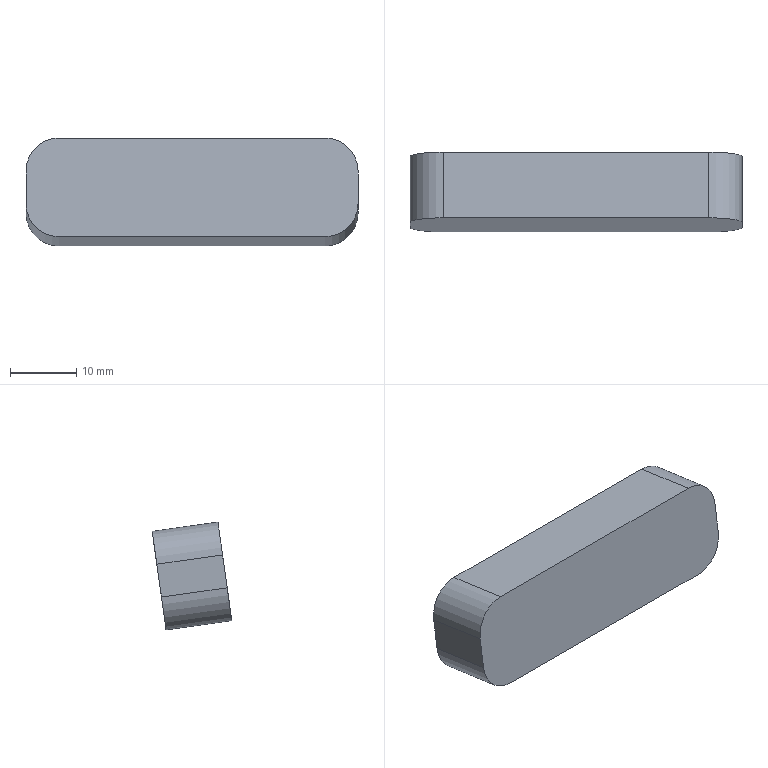Part | STEP file | SL2-MOLD_id6_xmt_txt | 1 solid | 10 faces | box 50 x 11.99 x 16.246 mm | volume 7285 mm3 | plane 6 | cylinder 4 | commonest cylinder face diameters 10 x4
STEP:
#1=CARTESIAN_POINT('',(25.,291.753,13.476));
#2=VERTEX_POINT('',#1);
#3=CARTESIAN_POINT('',(25.,291.057,8.524));
#4=VERTEX_POINT('',#3);
#5=CARTESIAN_POINT('',(25.,292.449,18.427));
#6=DIRECTION('',(0.,-0.1392,-0.9903));
#7=VECTOR('',#6,1.);
#8=LINE('',#5,#7);
#9=EDGE_CURVE('',#2,#4,#8,.T.);
#10=ORIENTED_EDGE('',*,*,#9,.F.);
#11=CARTESIAN_POINT('',(25.,281.851,14.867));
#12=VERTEX_POINT('',#11);
#13=CARTESIAN_POINT('',(25.,291.753,13.476));
#14=DIRECTION('',(0.,-0.9903,0.1392));
#15=VECTOR('',#14,1.);
#16=LINE('',#13,#15);
#17=EDGE_CURVE('',#2,#12,#16,.T.);
#18=ORIENTED_EDGE('',*,*,#17,.T.);
#19=CARTESIAN_POINT('',(25.,281.155,9.916));
#20=VERTEX_POINT('',#19);
#21=CARTESIAN_POINT('',(25.,282.547,19.819));
#22=DIRECTION('',(0.,-0.1392,-0.9903));
#23=VECTOR('',#22,1.);
#24=LINE('',#21,#23);
#25=EDGE_CURVE('',#12,#20,#24,.T.);
#26=ORIENTED_EDGE('',*,*,#25,.T.);
#27=CARTESIAN_POINT('',(25.,291.057,8.524));
#28=DIRECTION('',(0.,0.9903,-0.1392));
#29=VECTOR('',#28,1.);
#30=LINE('',#27,#29);
#31=EDGE_CURVE('',#20,#4,#30,.T.);
#32=ORIENTED_EDGE('',*,*,#31,.T.);
#33=EDGE_LOOP('',(#10,#18,#26,#32));
#34=FACE_OUTER_BOUND('',#33,.T.);
#35=CARTESIAN_POINT('',(25.,292.449,18.427));
#36=DIRECTION('',(-1.,0.,0.));
#37=DIRECTION('',(0.,0.,-1.));
#38=AXIS2_PLACEMENT_3D('',#35,#36,#37);
#39=PLANE('',#38);
#40=ADVANCED_FACE('',(#34),#39,.F.);
#41=CARTESIAN_POINT('',(20.,280.459,4.965));
#42=VERTEX_POINT('',#41);
#43=CARTESIAN_POINT('',(-20.,280.459,4.965));
#44=VERTEX_POINT('',#43);
#45=CARTESIAN_POINT('',(25.,280.459,4.965));
#46=DIRECTION('',(-1.,0.,0.));
#47=VECTOR('',#46,1.);
#48=LINE('',#45,#47);
#49=EDGE_CURVE('',#42,#44,#48,.T.);
#50=ORIENTED_EDGE('',*,*,#49,.T.);
#51=CARTESIAN_POINT('',(-20.,290.362,3.573));
#52=VERTEX_POINT('',#51);
#53=CARTESIAN_POINT('',(-20.,290.362,3.573));
#54=DIRECTION('',(0.,0.9903,-0.1392));
#55=VECTOR('',#54,1.);
#56=LINE('',#53,#55);
#57=EDGE_CURVE('',#44,#52,#56,.T.);
#58=ORIENTED_EDGE('',*,*,#57,.T.);
#59=CARTESIAN_POINT('',(20.,290.362,3.573));
#60=VERTEX_POINT('',#59);
#61=CARTESIAN_POINT('',(25.,290.362,3.573));
#62=DIRECTION('',(-1.,0.,0.));
#63=VECTOR('',#62,1.);
#64=LINE('',#61,#63);
#65=EDGE_CURVE('',#60,#52,#64,.T.);
#66=ORIENTED_EDGE('',*,*,#65,.F.);
#67=CARTESIAN_POINT('',(20.,290.362,3.573));
#68=DIRECTION('',(0.,-0.9903,0.1392));
#69=VECTOR('',#68,1.);
#70=LINE('',#67,#69);
#71=EDGE_CURVE('',#60,#42,#70,.T.);
#72=ORIENTED_EDGE('',*,*,#71,.T.);
#73=EDGE_LOOP('',(#50,#58,#66,#72));
#74=FACE_OUTER_BOUND('',#73,.T.);
#75=CARTESIAN_POINT('',(25.,290.362,3.573));
#76=DIRECTION('',(0.,0.1392,0.9903));
#77=DIRECTION('',(0.,-0.9903,0.1392));
#78=AXIS2_PLACEMENT_3D('',#75,#76,#77);
#79=PLANE('',#78);
#80=ADVANCED_FACE('',(#74),#79,.F.);
#81=CARTESIAN_POINT('',(-25.,281.155,9.916));
#82=VERTEX_POINT('',#81);
#83=CARTESIAN_POINT('',(-25.,281.851,14.867));
#84=VERTEX_POINT('',#83);
#85=CARTESIAN_POINT('',(-25.,280.459,4.965));
#86=DIRECTION('',(0.,0.1392,0.9903));
#87=VECTOR('',#86,1.);
#88=LINE('',#85,#87);
#89=EDGE_CURVE('',#82,#84,#88,.T.);
#90=ORIENTED_EDGE('',*,*,#89,.T.);
#91=CARTESIAN_POINT('',(-25.,291.753,13.476));
#92=VERTEX_POINT('',#91);
#93=CARTESIAN_POINT('',(-25.,291.753,13.476));
#94=DIRECTION('',(0.,0.9903,-0.1392));
#95=VECTOR('',#94,1.);
#96=LINE('',#93,#95);
#97=EDGE_CURVE('',#84,#92,#96,.T.);
#98=ORIENTED_EDGE('',*,*,#97,.T.);
#99=CARTESIAN_POINT('',(-25.,291.057,8.524));
#100=VERTEX_POINT('',#99);
#101=CARTESIAN_POINT('',(-25.,290.362,3.573));
#102=DIRECTION('',(0.,0.1392,0.9903));
#103=VECTOR('',#102,1.);
#104=LINE('',#101,#103);
#105=EDGE_CURVE('',#100,#92,#104,.T.);
#106=ORIENTED_EDGE('',*,*,#105,.F.);
#107=CARTESIAN_POINT('',(-25.,291.057,8.524));
#108=DIRECTION('',(0.,-0.9903,0.1392));
#109=VECTOR('',#108,1.);
#110=LINE('',#107,#109);
#111=EDGE_CURVE('',#100,#82,#110,.T.);
#112=ORIENTED_EDGE('',*,*,#111,.T.);
#113=EDGE_LOOP('',(#90,#98,#106,#112));
#114=FACE_OUTER_BOUND('',#113,.T.);
#115=CARTESIAN_POINT('',(-25.,290.362,3.573));
#116=DIRECTION('',(1.,0.,0.));
#117=DIRECTION('',(0.,0.,1.));
#118=AXIS2_PLACEMENT_3D('',#115,#116,#117);
#119=PLANE('',#118);
#120=ADVANCED_FACE('',(#114),#119,.F.);
#121=CARTESIAN_POINT('',(-20.,292.449,18.427));
#122=VERTEX_POINT('',#121);
#123=CARTESIAN_POINT('',(20.,292.449,18.427));
#124=VERTEX_POINT('',#123);
#125=CARTESIAN_POINT('',(-25.,292.449,18.427));
#126=DIRECTION('',(1.,0.,0.));
#127=VECTOR('',#126,1.);
#128=LINE('',#125,#127);
#129=EDGE_CURVE('',#122,#124,#128,.T.);
#130=ORIENTED_EDGE('',*,*,#129,.F.);
#131=CARTESIAN_POINT('',(-20.,282.547,19.819));
#132=VERTEX_POINT('',#131);
#133=CARTESIAN_POINT('',(-20.,292.449,18.427));
#134=DIRECTION('',(0.,-0.9903,0.1392));
#135=VECTOR('',#134,1.);
#136=LINE('',#133,#135);
#137=EDGE_CURVE('',#122,#132,#136,.T.);
#138=ORIENTED_EDGE('',*,*,#137,.T.);
#139=CARTESIAN_POINT('',(20.,282.547,19.819));
#140=VERTEX_POINT('',#139);
#141=CARTESIAN_POINT('',(-25.,282.547,19.819));
#142=DIRECTION('',(1.,0.,0.));
#143=VECTOR('',#142,1.);
#144=LINE('',#141,#143);
#145=EDGE_CURVE('',#132,#140,#144,.T.);
#146=ORIENTED_EDGE('',*,*,#145,.T.);
#147=CARTESIAN_POINT('',(20.,292.449,18.427));
#148=DIRECTION('',(0.,0.9903,-0.1392));
#149=VECTOR('',#148,1.);
#150=LINE('',#147,#149);
#151=EDGE_CURVE('',#140,#124,#150,.T.);
#152=ORIENTED_EDGE('',*,*,#151,.T.);
#153=EDGE_LOOP('',(#130,#138,#146,#152));
#154=FACE_OUTER_BOUND('',#153,.T.);
#155=CARTESIAN_POINT('',(-25.,292.449,18.427));
#156=DIRECTION('',(0.,-0.1392,-0.9903));
#157=DIRECTION('',(0.,0.9903,-0.1392));
#158=AXIS2_PLACEMENT_3D('',#155,#156,#157);
#159=PLANE('',#158);
#160=ADVANCED_FACE('',(#154),#159,.F.);
#161=ORIENTED_EDGE('',*,*,#105,.T.);
#162=CARTESIAN_POINT('',(-20.,291.753,13.476));
#163=DIRECTION('',(0.,0.9903,-0.1392));
#164=DIRECTION('',(0.,0.1392,0.9903));
#165=AXIS2_PLACEMENT_3D('',#162,#163,#164);
#166=CIRCLE('',#165,5.);
#167=EDGE_CURVE('',#92,#122,#166,.T.);
#168=ORIENTED_EDGE('',*,*,#167,.T.);
#169=ORIENTED_EDGE('',*,*,#129,.T.);
#170=CARTESIAN_POINT('',(20.,291.753,13.476));
#171=DIRECTION('',(0.,0.9903,-0.1392));
#172=DIRECTION('',(0.,0.1392,0.9903));
#173=AXIS2_PLACEMENT_3D('',#170,#171,#172);
#174=CIRCLE('',#173,5.);
#175=EDGE_CURVE('',#124,#2,#174,.T.);
#176=ORIENTED_EDGE('',*,*,#175,.T.);
#177=ORIENTED_EDGE('',*,*,#9,.T.);
#178=CARTESIAN_POINT('',(20.,291.057,8.524));
#179=DIRECTION('',(0.,0.9903,-0.1392));
#180=DIRECTION('',(0.,0.1392,0.9903));
#181=AXIS2_PLACEMENT_3D('',#178,#179,#180);
#182=CIRCLE('',#181,5.);
#183=EDGE_CURVE('',#4,#60,#182,.T.);
#184=ORIENTED_EDGE('',*,*,#183,.T.);
#185=ORIENTED_EDGE('',*,*,#65,.T.);
#186=CARTESIAN_POINT('',(-20.,291.057,8.524));
#187=DIRECTION('',(0.,0.9903,-0.1392));
#188=DIRECTION('',(0.,0.1392,0.9903));
#189=AXIS2_PLACEMENT_3D('',#186,#187,#188);
#190=CIRCLE('',#189,5.);
#191=EDGE_CURVE('',#52,#100,#190,.T.);
#192=ORIENTED_EDGE('',*,*,#191,.T.);
#193=EDGE_LOOP('',(#161,#168,#169,#176,#177,#184,#185,#192));
#194=FACE_OUTER_BOUND('',#193,.T.);
#195=CARTESIAN_POINT('',(-175.,287.552,-16.422));
#196=DIRECTION('',(0.,0.9903,-0.1392));
#197=DIRECTION('',(0.,0.1392,0.9903));
#198=AXIS2_PLACEMENT_3D('',#195,#196,#197);
#199=PLANE('',#198);
#200=ADVANCED_FACE('',(#194),#199,.T.);
#201=ORIENTED_EDGE('',*,*,#145,.F.);
#202=CARTESIAN_POINT('',(-20.,281.851,14.867));
#203=DIRECTION('',(0.,-0.9903,0.1392));
#204=DIRECTION('',(0.,0.1392,0.9903));
#205=AXIS2_PLACEMENT_3D('',#202,#203,#204);
#206=CIRCLE('',#205,5.);
#207=EDGE_CURVE('',#132,#84,#206,.T.);
#208=ORIENTED_EDGE('',*,*,#207,.T.);
#209=ORIENTED_EDGE('',*,*,#89,.F.);
#210=CARTESIAN_POINT('',(-20.,281.155,9.916));
#211=DIRECTION('',(0.,-0.9903,0.1392));
#212=DIRECTION('',(0.,0.1392,0.9903));
#213=AXIS2_PLACEMENT_3D('',#210,#211,#212);
#214=CIRCLE('',#213,5.);
#215=EDGE_CURVE('',#82,#44,#214,.T.);
#216=ORIENTED_EDGE('',*,*,#215,.T.);
#217=ORIENTED_EDGE('',*,*,#49,.F.);
#218=CARTESIAN_POINT('',(20.,281.155,9.916));
#219=DIRECTION('',(0.,-0.9903,0.1392));
#220=DIRECTION('',(0.,0.1392,0.9903));
#221=AXIS2_PLACEMENT_3D('',#218,#219,#220);
#222=CIRCLE('',#221,5.);
#223=EDGE_CURVE('',#42,#20,#222,.T.);
#224=ORIENTED_EDGE('',*,*,#223,.T.);
#225=ORIENTED_EDGE('',*,*,#25,.F.);
#226=CARTESIAN_POINT('',(20.,281.851,14.867));
#227=DIRECTION('',(0.,-0.9903,0.1392));
#228=DIRECTION('',(0.,0.1392,0.9903));
#229=AXIS2_PLACEMENT_3D('',#226,#227,#228);
#230=CIRCLE('',#229,5.);
#231=EDGE_CURVE('',#12,#140,#230,.T.);
#232=ORIENTED_EDGE('',*,*,#231,.T.);
#233=EDGE_LOOP('',(#201,#208,#209,#216,#217,#224,#225,#232));
#234=FACE_OUTER_BOUND('',#233,.T.);
#235=CARTESIAN_POINT('',(-175.,277.649,-15.03));
#236=DIRECTION('',(0.,0.9903,-0.1392));
#237=DIRECTION('',(0.,0.1392,0.9903));
#238=AXIS2_PLACEMENT_3D('',#235,#236,#237);
#239=PLANE('',#238);
#240=ADVANCED_FACE('',(#234),#239,.F.);
#241=ORIENTED_EDGE('',*,*,#167,.F.);
#242=ORIENTED_EDGE('',*,*,#97,.F.);
#243=ORIENTED_EDGE('',*,*,#207,.F.);
#244=ORIENTED_EDGE('',*,*,#137,.F.);
#245=EDGE_LOOP('',(#241,#242,#243,#244));
#246=FACE_OUTER_BOUND('',#245,.T.);
#247=CARTESIAN_POINT('',(-20.,291.753,13.476));
#248=DIRECTION('',(0.,-0.9903,0.1392));
#249=DIRECTION('',(0.,-0.1392,-0.9903));
#250=AXIS2_PLACEMENT_3D('',#247,#248,#249);
#251=CYLINDRICAL_SURFACE('',#250,5.);
#252=ADVANCED_FACE('',(#246),#251,.T.);
#253=ORIENTED_EDGE('',*,*,#175,.F.);
#254=ORIENTED_EDGE('',*,*,#151,.F.);
#255=ORIENTED_EDGE('',*,*,#231,.F.);
#256=ORIENTED_EDGE('',*,*,#17,.F.);
#257=EDGE_LOOP('',(#253,#254,#255,#256));
#258=FACE_OUTER_BOUND('',#257,.T.);
#259=CARTESIAN_POINT('',(20.,291.753,13.476));
#260=DIRECTION('',(0.,-0.9903,0.1392));
#261=DIRECTION('',(0.,-0.1392,-0.9903));
#262=AXIS2_PLACEMENT_3D('',#259,#260,#261);
#263=CYLINDRICAL_SURFACE('',#262,5.);
#264=ADVANCED_FACE('',(#258),#263,.T.);
#265=ORIENTED_EDGE('',*,*,#191,.F.);
#266=ORIENTED_EDGE('',*,*,#57,.F.);
#267=ORIENTED_EDGE('',*,*,#215,.F.);
#268=ORIENTED_EDGE('',*,*,#111,.F.);
#269=EDGE_LOOP('',(#265,#266,#267,#268));
#270=FACE_OUTER_BOUND('',#269,.T.);
#271=CARTESIAN_POINT('',(-20.,291.057,8.524));
#272=DIRECTION('',(0.,-0.9903,0.1392));
#273=DIRECTION('',(0.,-0.1392,-0.9903));
#274=AXIS2_PLACEMENT_3D('',#271,#272,#273);
#275=CYLINDRICAL_SURFACE('',#274,5.);
#276=ADVANCED_FACE('',(#270),#275,.T.);
#277=ORIENTED_EDGE('',*,*,#183,.F.);
#278=ORIENTED_EDGE('',*,*,#31,.F.);
#279=ORIENTED_EDGE('',*,*,#223,.F.);
#280=ORIENTED_EDGE('',*,*,#71,.F.);
#281=EDGE_LOOP('',(#277,#278,#279,#280));
#282=FACE_OUTER_BOUND('',#281,.T.);
#283=CARTESIAN_POINT('',(20.,291.057,8.524));
#284=DIRECTION('',(0.,-0.9903,0.1392));
#285=DIRECTION('',(0.,-0.1392,-0.9903));
#286=AXIS2_PLACEMENT_3D('',#283,#284,#285);
#287=CYLINDRICAL_SURFACE('',#286,5.);
#288=ADVANCED_FACE('',(#282),#287,.T.);
#289=CLOSED_SHELL('',(#40,#80,#120,#160,#200,#240,#252,#264,#276,#288));
#290=MANIFOLD_SOLID_BREP('',#289);
#291=(LENGTH_UNIT()NAMED_UNIT(*)SI_UNIT(.MILLI.,.METRE.));
#292=UNCERTAINTY_MEASURE_WITH_UNIT(LENGTH_MEASURE(0.00002),#291,'','');
#293=(NAMED_UNIT(*)PLANE_ANGLE_UNIT()SI_UNIT($,.RADIAN.));
#294=PLANE_ANGLE_MEASURE_WITH_UNIT(PLANE_ANGLE_MEASURE(0.01745),#293);
#295=DIMENSIONAL_EXPONENTS(0.,0.,0.,0.,0.,0.,0.);
#296=(CONVERSION_BASED_UNIT('DEGREE',#294)NAMED_UNIT(#295)PLANE_ANGLE_UNIT());
#297=(NAMED_UNIT(*)SI_UNIT($,.STERADIAN.)SOLID_ANGLE_UNIT());
#298=(GEOMETRIC_REPRESENTATION_CONTEXT(3)GLOBAL_UNCERTAINTY_ASSIGNED_CONTEXT((#292))GLOBAL_UNIT_ASSIGNED_CONTEXT((#291,#296,#297))REPRESENTATION_CONTEXT('',''));
#299=ADVANCED_BREP_SHAPE_REPRESENTATION('',(#290),#298);